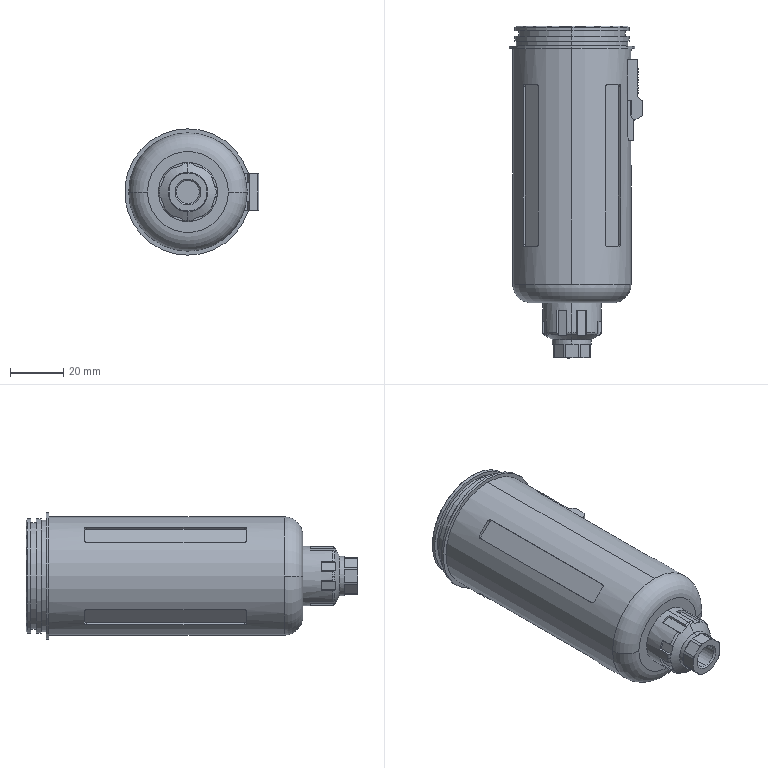Part | SolidWorks | features BaseBody 1 | 1 solid | 224 faces | box 50.45 x 124.7 x 47.5 mm | volume 63233 mm3 | plane 149 | cylinder 47 | torus 22 | cone 6 | commonest cylinder face diameters 2 x20 4 x5 43 x4 8.566 x2 14.823 x2 22.235 x2